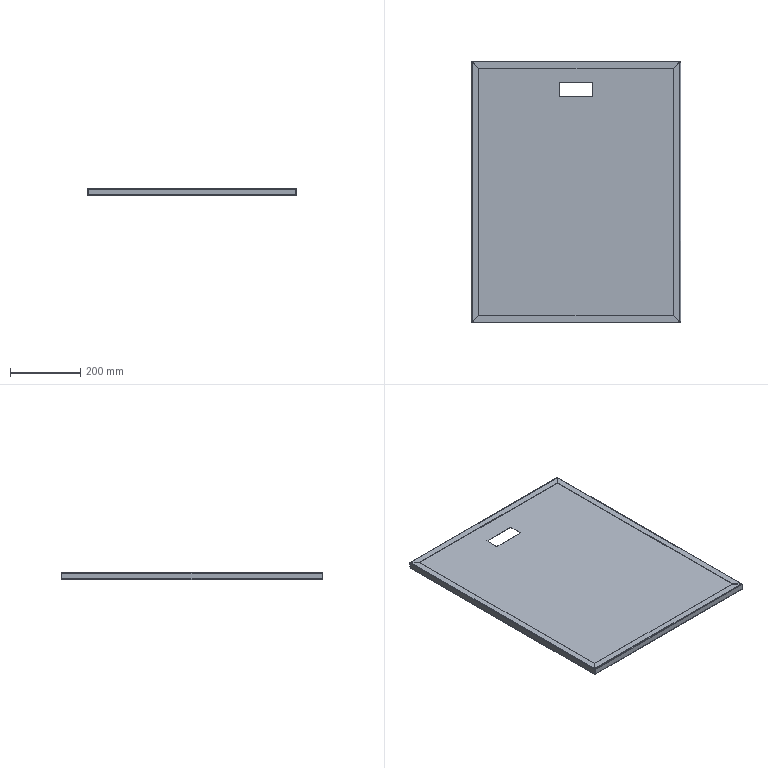Part | SolidWorks | features EdgeFlange 2, FlatPattern 1, ICE 1, SMBaseFlange 1, SheetMetal 1 | 1 solid | 74 faces | box 597 x 747 x 20 mm | volume 645008 mm3 | plane 42 | spline 16 | cylinder 16 | commonest cylinder face diameters 2 x8 4.4 x8